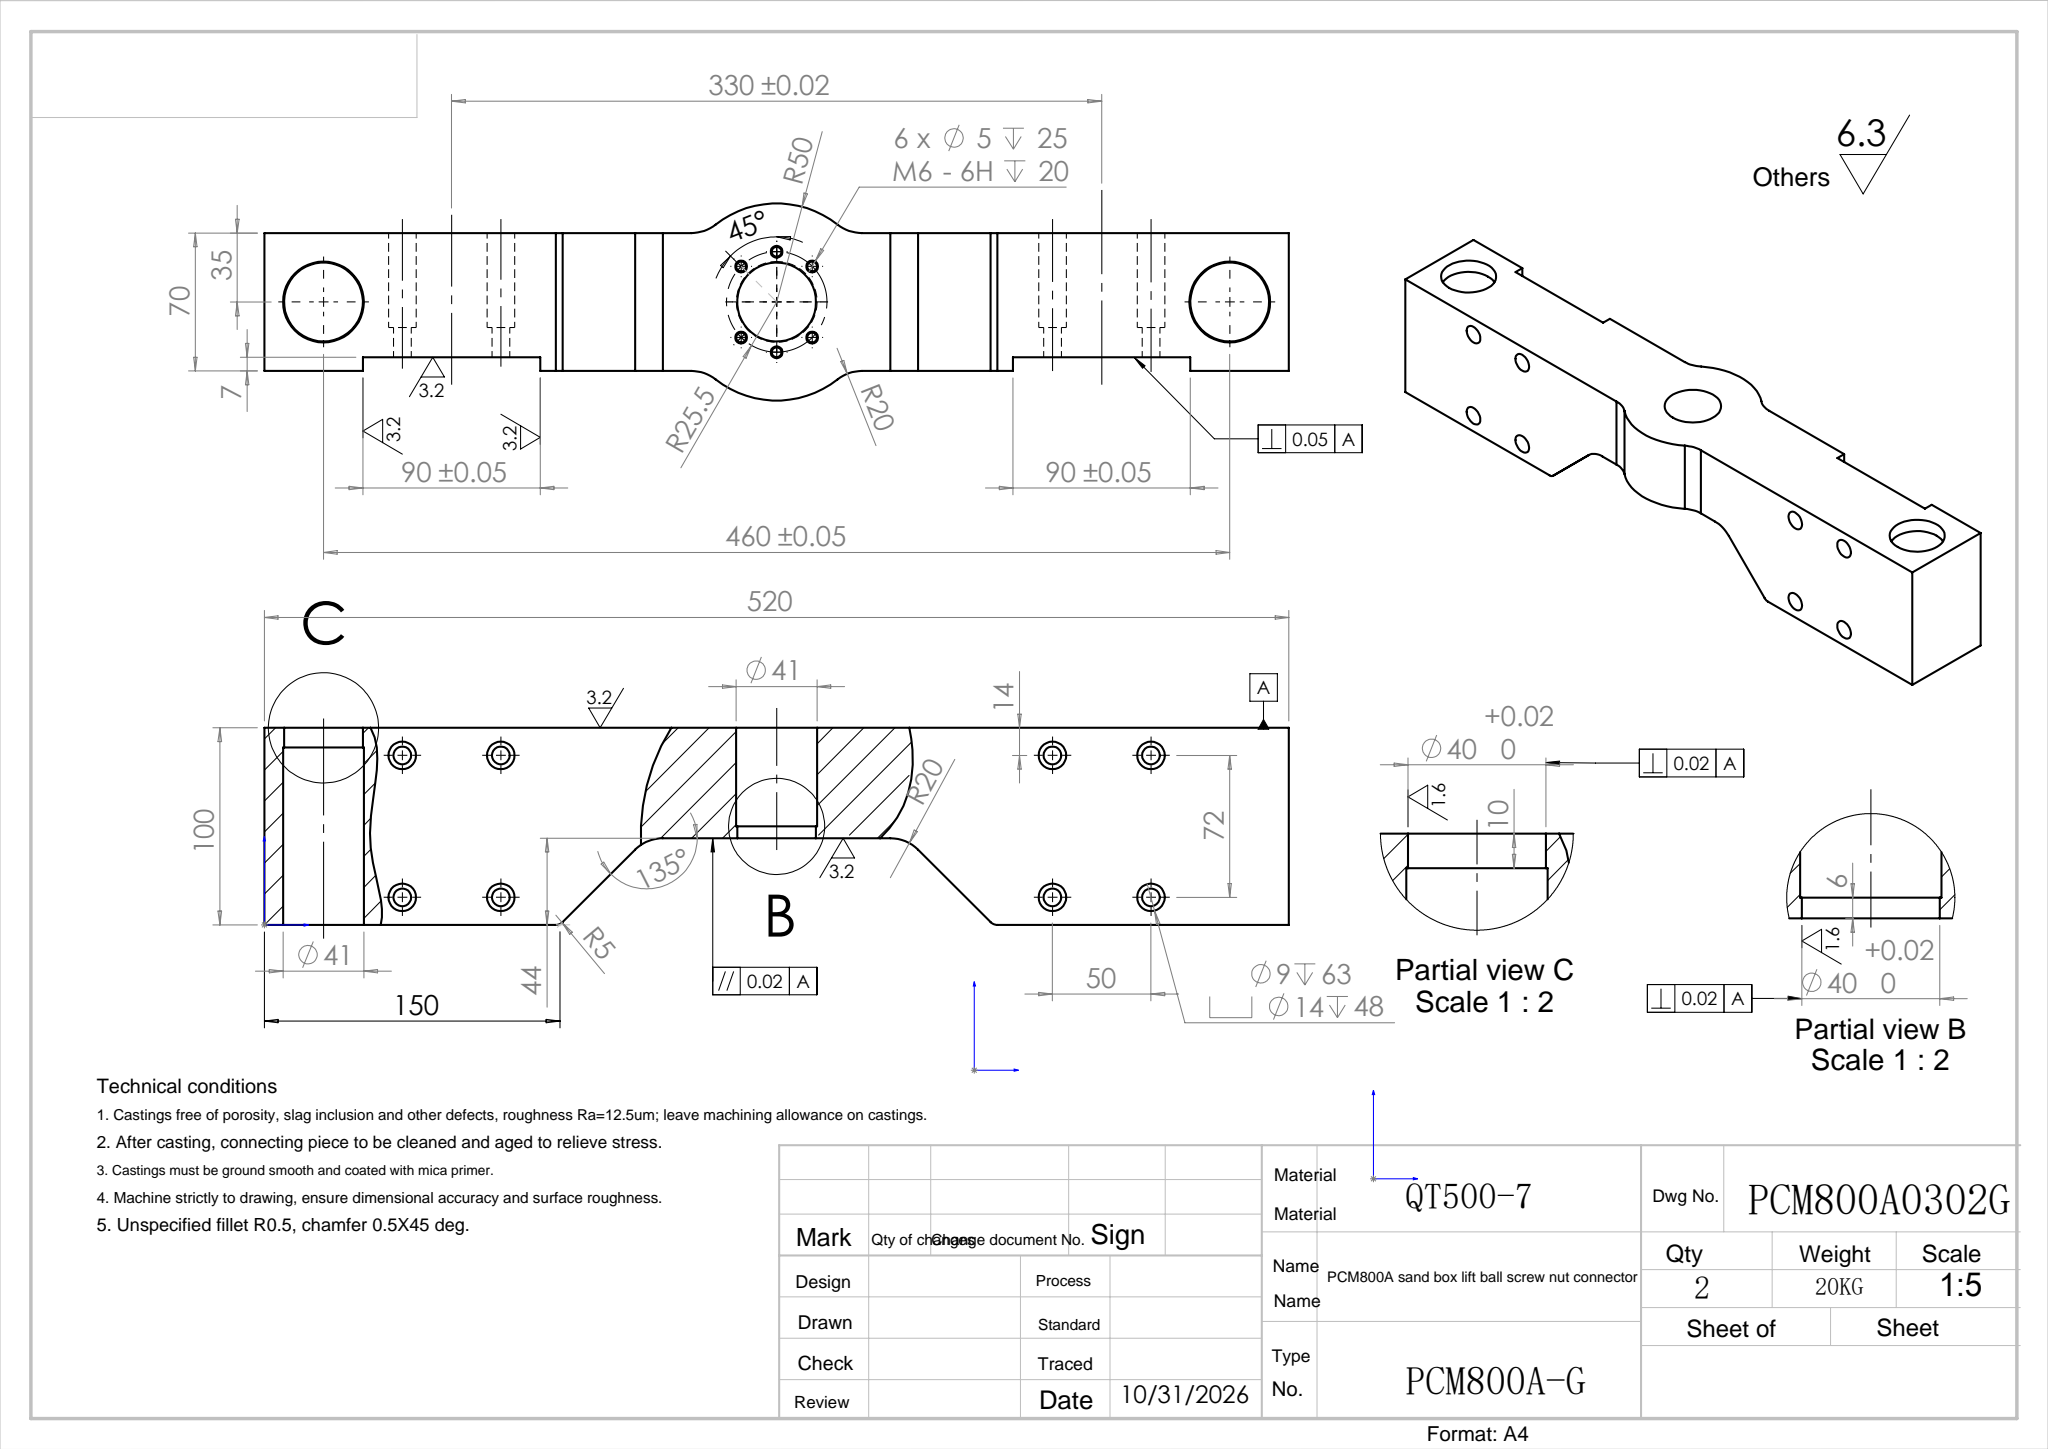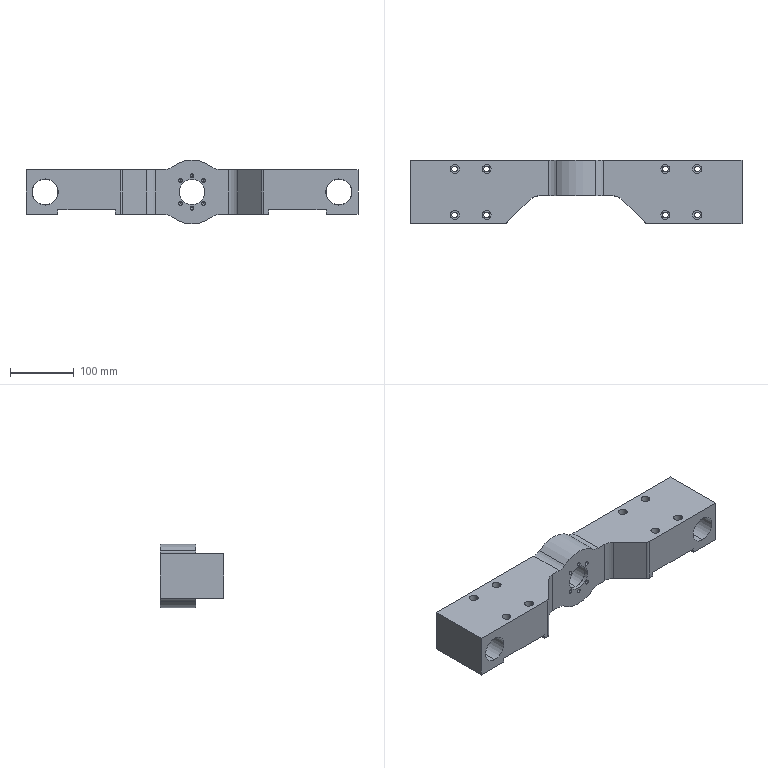Part | SolidWorks | features Cut 5, Attribute 4, ICE 3, Extrusion 1, Fillet 1, HoleWzd 1, MirrorPattern 1 | 1 solid | 128 faces | box 520 x 100 x 100 mm | volume 2650054 mm3 | cylinder 79 | plane 37 | cone 12 | commonest cylinder face diameters 9 x16 14 x16 5 x12 6 x12 40 x12 41 x6